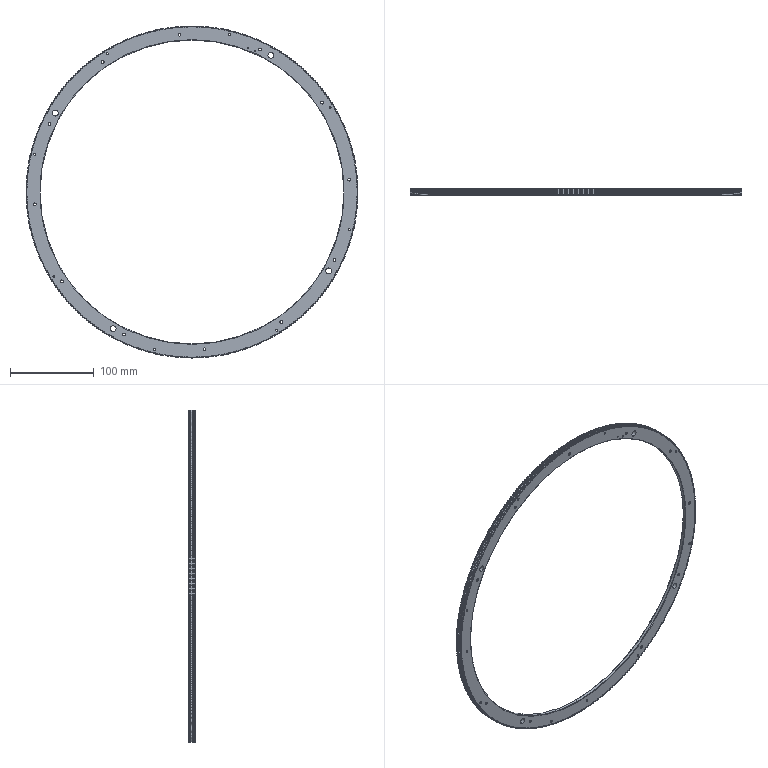Part | NX | features BREP 1 | 1 solid | 3349 faces | volume 89680 mm3 | cylinder 3096 | cone 150 | plane 103 | commonest cylinder face diameters 0.5 x1022 3.04 x884 1.7 x543 396.69 x416 10 x60 4 x50